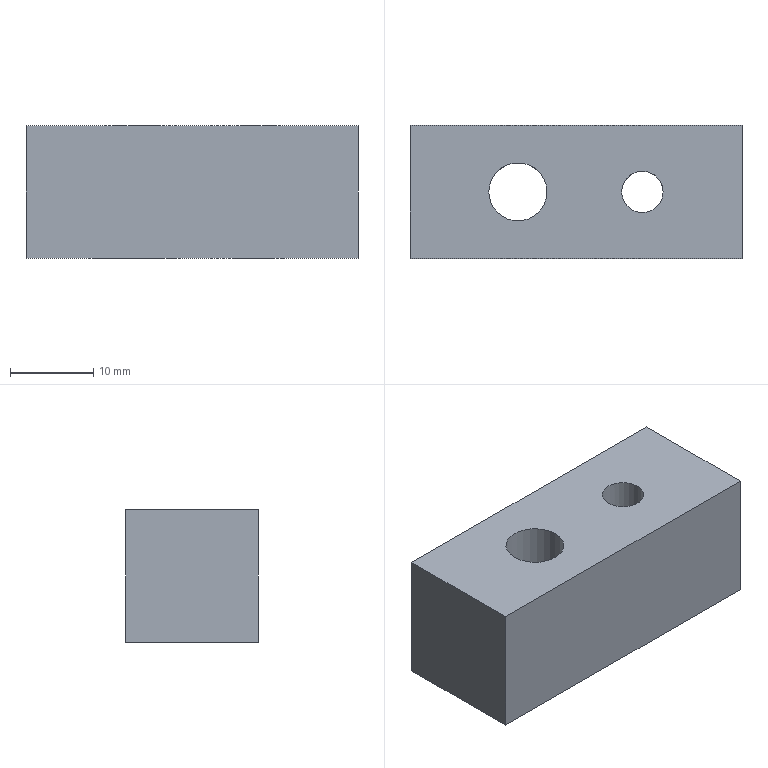Part | STEP file | gslz 2016.10.28-6_id238_x_t | 1 solid | 11 faces | box 40 x 16 x 16 mm | volume 8856 mm3 | plane 7 | cylinder 3 | cone 1 | commonest cylinder face diameters 5 x1 7 x1 11 x1
STEP:
#1=CARTESIAN_POINT('',(8.,158.,121.992));
#2=VERTEX_POINT('',#1);
#3=CARTESIAN_POINT('',(8.,155.,121.992));
#4=DIRECTION('',(0.,0.,1.));
#5=DIRECTION('',(0.,1.,0.));
#6=AXIS2_PLACEMENT_3D('',#3,#4,#5);
#7=CIRCLE('',#6,3.);
#8=EDGE_CURVE('',#2,#2,#7,.T.);
#9=ORIENTED_EDGE('',*,*,#8,.T.);
#10=EDGE_LOOP('',(#9));
#11=FACE_BOUND('',#10,.T.);
#12=CARTESIAN_POINT('',(-20.,147.,121.992));
#13=VERTEX_POINT('',#12);
#14=CARTESIAN_POINT('',(-20.,163.,121.992));
#15=VERTEX_POINT('',#14);
#16=CARTESIAN_POINT('',(-20.,147.,121.992));
#17=DIRECTION('',(0.,1.,0.));
#18=VECTOR('',#17,1.);
#19=LINE('',#16,#18);
#20=EDGE_CURVE('',#13,#15,#19,.T.);
#21=ORIENTED_EDGE('',*,*,#20,.T.);
#22=CARTESIAN_POINT('',(20.,163.,121.992));
#23=VERTEX_POINT('',#22);
#24=CARTESIAN_POINT('',(-20.,163.,121.992));
#25=DIRECTION('',(1.,0.,0.));
#26=VECTOR('',#25,1.);
#27=LINE('',#24,#26);
#28=EDGE_CURVE('',#15,#23,#27,.T.);
#29=ORIENTED_EDGE('',*,*,#28,.T.);
#30=CARTESIAN_POINT('',(20.,147.,121.992));
#31=VERTEX_POINT('',#30);
#32=CARTESIAN_POINT('',(20.,163.,121.992));
#33=DIRECTION('',(0.,-1.,0.));
#34=VECTOR('',#33,1.);
#35=LINE('',#32,#34);
#36=EDGE_CURVE('',#23,#31,#35,.T.);
#37=ORIENTED_EDGE('',*,*,#36,.T.);
#38=CARTESIAN_POINT('',(10.,147.,121.992));
#39=DIRECTION('',(-1.,0.,0.));
#40=VECTOR('',#39,1.);
#41=LINE('',#38,#40);
#42=EDGE_CURVE('',#31,#13,#41,.T.);
#43=ORIENTED_EDGE('',*,*,#42,.T.);
#44=EDGE_LOOP('',(#21,#29,#37,#43));
#45=FACE_BOUND('',#44,.T.);
#46=CARTESIAN_POINT('',(-1.5,155.,121.992));
#47=VERTEX_POINT('',#46);
#48=CARTESIAN_POINT('',(-7.,155.,121.992));
#49=DIRECTION('',(0.,0.,-1.));
#50=DIRECTION('',(1.,0.,0.));
#51=AXIS2_PLACEMENT_3D('',#48,#49,#50);
#52=CIRCLE('',#51,5.5);
#53=EDGE_CURVE('',#47,#47,#52,.T.);
#54=ORIENTED_EDGE('',*,*,#53,.F.);
#55=EDGE_LOOP('',(#54));
#56=FACE_BOUND('',#55,.T.);
#57=CARTESIAN_POINT('',(-20.,147.,121.992));
#58=DIRECTION('',(0.,0.,-1.));
#59=DIRECTION('',(-1.,0.,0.));
#60=AXIS2_PLACEMENT_3D('',#57,#58,#59);
#61=PLANE('',#60);
#62=ADVANCED_FACE('',(#11,#45,#56),#61,.T.);
#63=CARTESIAN_POINT('',(-3.5,155.,129.992));
#64=VERTEX_POINT('',#63);
#65=CARTESIAN_POINT('',(-7.,155.,129.992));
#66=DIRECTION('',(0.,0.,-1.));
#67=DIRECTION('',(1.,0.,0.));
#68=AXIS2_PLACEMENT_3D('',#65,#66,#67);
#69=CIRCLE('',#68,3.5);
#70=EDGE_CURVE('',#64,#64,#69,.T.);
#71=ORIENTED_EDGE('',*,*,#70,.F.);
#72=EDGE_LOOP('',(#71));
#73=FACE_BOUND('',#72,.T.);
#74=CARTESIAN_POINT('',(-1.5,155.,129.992));
#75=VERTEX_POINT('',#74);
#76=CARTESIAN_POINT('',(-7.,155.,129.992));
#77=DIRECTION('',(0.,0.,-1.));
#78=DIRECTION('',(1.,0.,0.));
#79=AXIS2_PLACEMENT_3D('',#76,#77,#78);
#80=CIRCLE('',#79,5.5);
#81=EDGE_CURVE('',#75,#75,#80,.T.);
#82=ORIENTED_EDGE('',*,*,#81,.T.);
#83=EDGE_LOOP('',(#82));
#84=FACE_BOUND('',#83,.T.);
#85=CARTESIAN_POINT('',(-7.,155.,129.992));
#86=DIRECTION('',(0.,0.,-1.));
#87=DIRECTION('',(-1.,0.,0.));
#88=AXIS2_PLACEMENT_3D('',#85,#86,#87);
#89=PLANE('',#88);
#90=ADVANCED_FACE('',(#73,#84),#89,.T.);
#91=CARTESIAN_POINT('',(8.,157.5,122.492));
#92=VERTEX_POINT('',#91);
#93=CARTESIAN_POINT('',(8.,155.,122.492));
#94=DIRECTION('',(0.,0.,-1.));
#95=DIRECTION('',(0.,1.,0.));
#96=AXIS2_PLACEMENT_3D('',#93,#94,#95);
#97=CIRCLE('',#96,2.5);
#98=EDGE_CURVE('',#92,#92,#97,.T.);
#99=ORIENTED_EDGE('',*,*,#98,.T.);
#100=EDGE_LOOP('',(#99));
#101=FACE_BOUND('',#100,.T.);
#102=CARTESIAN_POINT('',(10.5,155.,137.992));
#103=VERTEX_POINT('',#102);
#104=CARTESIAN_POINT('',(8.,155.,137.992));
#105=DIRECTION('',(0.,0.,1.));
#106=DIRECTION('',(1.,0.,0.));
#107=AXIS2_PLACEMENT_3D('',#104,#105,#106);
#108=CIRCLE('',#107,2.5);
#109=EDGE_CURVE('',#103,#103,#108,.T.);
#110=ORIENTED_EDGE('',*,*,#109,.T.);
#111=EDGE_LOOP('',(#110));
#112=FACE_BOUND('',#111,.T.);
#113=CARTESIAN_POINT('',(8.,155.,105.992));
#114=DIRECTION('',(0.,0.,1.));
#115=DIRECTION('',(1.,0.,0.));
#116=AXIS2_PLACEMENT_3D('',#113,#114,#115);
#117=CYLINDRICAL_SURFACE('',#116,2.5);
#118=ADVANCED_FACE('',(#101,#112),#117,.F.);
#119=ORIENTED_EDGE('',*,*,#36,.F.);
#120=CARTESIAN_POINT('',(20.,163.,137.992));
#121=VERTEX_POINT('',#120);
#122=CARTESIAN_POINT('',(20.,163.,121.992));
#123=DIRECTION('',(0.,0.,-1.));
#124=VECTOR('',#123,1.);
#125=LINE('',#122,#124);
#126=EDGE_CURVE('',#121,#23,#125,.T.);
#127=ORIENTED_EDGE('',*,*,#126,.F.);
#128=CARTESIAN_POINT('',(20.,147.,137.992));
#129=VERTEX_POINT('',#128);
#130=CARTESIAN_POINT('',(20.,163.,137.992));
#131=DIRECTION('',(0.,-1.,0.));
#132=VECTOR('',#131,1.);
#133=LINE('',#130,#132);
#134=EDGE_CURVE('',#121,#129,#133,.T.);
#135=ORIENTED_EDGE('',*,*,#134,.T.);
#136=CARTESIAN_POINT('',(20.,147.,121.992));
#137=DIRECTION('',(0.,0.,-1.));
#138=VECTOR('',#137,1.);
#139=LINE('',#136,#138);
#140=EDGE_CURVE('',#129,#31,#139,.T.);
#141=ORIENTED_EDGE('',*,*,#140,.T.);
#142=EDGE_LOOP('',(#119,#127,#135,#141));
#143=FACE_OUTER_BOUND('',#142,.T.);
#144=CARTESIAN_POINT('',(20.,163.,121.992));
#145=DIRECTION('',(-1.,0.,0.));
#146=DIRECTION('',(0.,0.,1.));
#147=AXIS2_PLACEMENT_3D('',#144,#145,#146);
#148=PLANE('',#147);
#149=ADVANCED_FACE('',(#143),#148,.F.);
#150=ORIENTED_EDGE('',*,*,#42,.F.);
#151=ORIENTED_EDGE('',*,*,#140,.F.);
#152=CARTESIAN_POINT('',(-20.,147.,137.992));
#153=VERTEX_POINT('',#152);
#154=CARTESIAN_POINT('',(10.,147.,137.992));
#155=DIRECTION('',(-1.,0.,0.));
#156=VECTOR('',#155,1.);
#157=LINE('',#154,#156);
#158=EDGE_CURVE('',#129,#153,#157,.T.);
#159=ORIENTED_EDGE('',*,*,#158,.T.);
#160=CARTESIAN_POINT('',(-20.,147.,121.992));
#161=DIRECTION('',(0.,0.,-1.));
#162=VECTOR('',#161,1.);
#163=LINE('',#160,#162);
#164=EDGE_CURVE('',#153,#13,#163,.T.);
#165=ORIENTED_EDGE('',*,*,#164,.T.);
#166=EDGE_LOOP('',(#150,#151,#159,#165));
#167=FACE_OUTER_BOUND('',#166,.T.);
#168=CARTESIAN_POINT('',(10.,147.,121.992));
#169=DIRECTION('',(0.,1.,0.));
#170=DIRECTION('',(0.,0.,-1.));
#171=AXIS2_PLACEMENT_3D('',#168,#169,#170);
#172=PLANE('',#171);
#173=ADVANCED_FACE('',(#167),#172,.F.);
#174=CARTESIAN_POINT('',(-20.,163.,137.992));
#175=VERTEX_POINT('',#174);
#176=CARTESIAN_POINT('',(-20.,147.,137.992));
#177=DIRECTION('',(0.,1.,0.));
#178=VECTOR('',#177,1.);
#179=LINE('',#176,#178);
#180=EDGE_CURVE('',#153,#175,#179,.T.);
#181=ORIENTED_EDGE('',*,*,#180,.T.);
#182=CARTESIAN_POINT('',(-20.,163.,121.992));
#183=DIRECTION('',(0.,0.,-1.));
#184=VECTOR('',#183,1.);
#185=LINE('',#182,#184);
#186=EDGE_CURVE('',#175,#15,#185,.T.);
#187=ORIENTED_EDGE('',*,*,#186,.T.);
#188=ORIENTED_EDGE('',*,*,#20,.F.);
#189=ORIENTED_EDGE('',*,*,#164,.F.);
#190=EDGE_LOOP('',(#181,#187,#188,#189));
#191=FACE_OUTER_BOUND('',#190,.T.);
#192=CARTESIAN_POINT('',(-20.,147.,121.992));
#193=DIRECTION('',(1.,0.,0.));
#194=DIRECTION('',(0.,0.,-1.));
#195=AXIS2_PLACEMENT_3D('',#192,#193,#194);
#196=PLANE('',#195);
#197=ADVANCED_FACE('',(#191),#196,.F.);
#198=ORIENTED_EDGE('',*,*,#28,.F.);
#199=ORIENTED_EDGE('',*,*,#186,.F.);
#200=CARTESIAN_POINT('',(-20.,163.,137.992));
#201=DIRECTION('',(1.,0.,0.));
#202=VECTOR('',#201,1.);
#203=LINE('',#200,#202);
#204=EDGE_CURVE('',#175,#121,#203,.T.);
#205=ORIENTED_EDGE('',*,*,#204,.T.);
#206=ORIENTED_EDGE('',*,*,#126,.T.);
#207=EDGE_LOOP('',(#198,#199,#205,#206));
#208=FACE_OUTER_BOUND('',#207,.T.);
#209=CARTESIAN_POINT('',(-20.,163.,121.992));
#210=DIRECTION('',(0.,-1.,0.));
#211=DIRECTION('',(0.,0.,1.));
#212=AXIS2_PLACEMENT_3D('',#209,#210,#211);
#213=PLANE('',#212);
#214=ADVANCED_FACE('',(#208),#213,.F.);
#215=CARTESIAN_POINT('',(-3.5,155.,137.992));
#216=VERTEX_POINT('',#215);
#217=CARTESIAN_POINT('',(-7.,155.,137.992));
#218=DIRECTION('',(0.,0.,1.));
#219=DIRECTION('',(1.,0.,0.));
#220=AXIS2_PLACEMENT_3D('',#217,#218,#219);
#221=CIRCLE('',#220,3.5);
#222=EDGE_CURVE('',#216,#216,#221,.T.);
#223=ORIENTED_EDGE('',*,*,#222,.T.);
#224=EDGE_LOOP('',(#223));
#225=FACE_BOUND('',#224,.T.);
#226=ORIENTED_EDGE('',*,*,#70,.T.);
#227=EDGE_LOOP('',(#226));
#228=FACE_BOUND('',#227,.T.);
#229=CARTESIAN_POINT('',(-7.,155.,105.992));
#230=DIRECTION('',(0.,0.,1.));
#231=DIRECTION('',(1.,0.,0.));
#232=AXIS2_PLACEMENT_3D('',#229,#230,#231);
#233=CYLINDRICAL_SURFACE('',#232,3.5);
#234=ADVANCED_FACE('',(#225,#228),#233,.F.);
#235=ORIENTED_EDGE('',*,*,#222,.F.);
#236=EDGE_LOOP('',(#235));
#237=FACE_BOUND('',#236,.T.);
#238=ORIENTED_EDGE('',*,*,#204,.F.);
#239=ORIENTED_EDGE('',*,*,#180,.F.);
#240=ORIENTED_EDGE('',*,*,#158,.F.);
#241=ORIENTED_EDGE('',*,*,#134,.F.);
#242=EDGE_LOOP('',(#238,#239,#240,#241));
#243=FACE_BOUND('',#242,.T.);
#244=ORIENTED_EDGE('',*,*,#109,.F.);
#245=EDGE_LOOP('',(#244));
#246=FACE_BOUND('',#245,.T.);
#247=CARTESIAN_POINT('',(-20.,147.,137.992));
#248=DIRECTION('',(0.,0.,-1.));
#249=DIRECTION('',(-1.,0.,0.));
#250=AXIS2_PLACEMENT_3D('',#247,#248,#249);
#251=PLANE('',#250);
#252=ADVANCED_FACE('',(#237,#243,#246),#251,.F.);
#253=ORIENTED_EDGE('',*,*,#81,.F.);
#254=EDGE_LOOP('',(#253));
#255=FACE_BOUND('',#254,.T.);
#256=ORIENTED_EDGE('',*,*,#53,.T.);
#257=EDGE_LOOP('',(#256));
#258=FACE_BOUND('',#257,.T.);
#259=CARTESIAN_POINT('',(-7.,155.,129.992));
#260=DIRECTION('',(0.,0.,-1.));
#261=DIRECTION('',(-1.,0.,0.));
#262=AXIS2_PLACEMENT_3D('',#259,#260,#261);
#263=CYLINDRICAL_SURFACE('',#262,5.5);
#264=ADVANCED_FACE('',(#255,#258),#263,.F.);
#265=ORIENTED_EDGE('',*,*,#98,.F.);
#266=EDGE_LOOP('',(#265));
#267=FACE_BOUND('',#266,.T.);
#268=ORIENTED_EDGE('',*,*,#8,.F.);
#269=EDGE_LOOP('',(#268));
#270=FACE_BOUND('',#269,.T.);
#271=CARTESIAN_POINT('',(8.,155.,121.992));
#272=DIRECTION('',(0.,0.,-1.));
#273=DIRECTION('',(0.,1.,0.));
#274=AXIS2_PLACEMENT_3D('',#271,#272,#273);
#275=CONICAL_SURFACE('',#274,3.,45.);
#276=ADVANCED_FACE('',(#267,#270),#275,.F.);
#277=CLOSED_SHELL('',(#62,#90,#118,#149,#173,#197,#214,#234,#252,#264,#276));
#278=MANIFOLD_SOLID_BREP('',#277);
#279=(LENGTH_UNIT()NAMED_UNIT(*)SI_UNIT(.MILLI.,.METRE.));
#280=UNCERTAINTY_MEASURE_WITH_UNIT(LENGTH_MEASURE(0.00002),#279,'','');
#281=(NAMED_UNIT(*)PLANE_ANGLE_UNIT()SI_UNIT($,.RADIAN.));
#282=PLANE_ANGLE_MEASURE_WITH_UNIT(PLANE_ANGLE_MEASURE(0.01745),#281);
#283=DIMENSIONAL_EXPONENTS(0.,0.,0.,0.,0.,0.,0.);
#284=(CONVERSION_BASED_UNIT('DEGREE',#282)NAMED_UNIT(#283)PLANE_ANGLE_UNIT());
#285=(NAMED_UNIT(*)SI_UNIT($,.STERADIAN.)SOLID_ANGLE_UNIT());
#286=(GEOMETRIC_REPRESENTATION_CONTEXT(3)GLOBAL_UNCERTAINTY_ASSIGNED_CONTEXT((#280))GLOBAL_UNIT_ASSIGNED_CONTEXT((#279,#284,#285))REPRESENTATION_CONTEXT('',''));
#287=ADVANCED_BREP_SHAPE_REPRESENTATION('',(#278),#286);